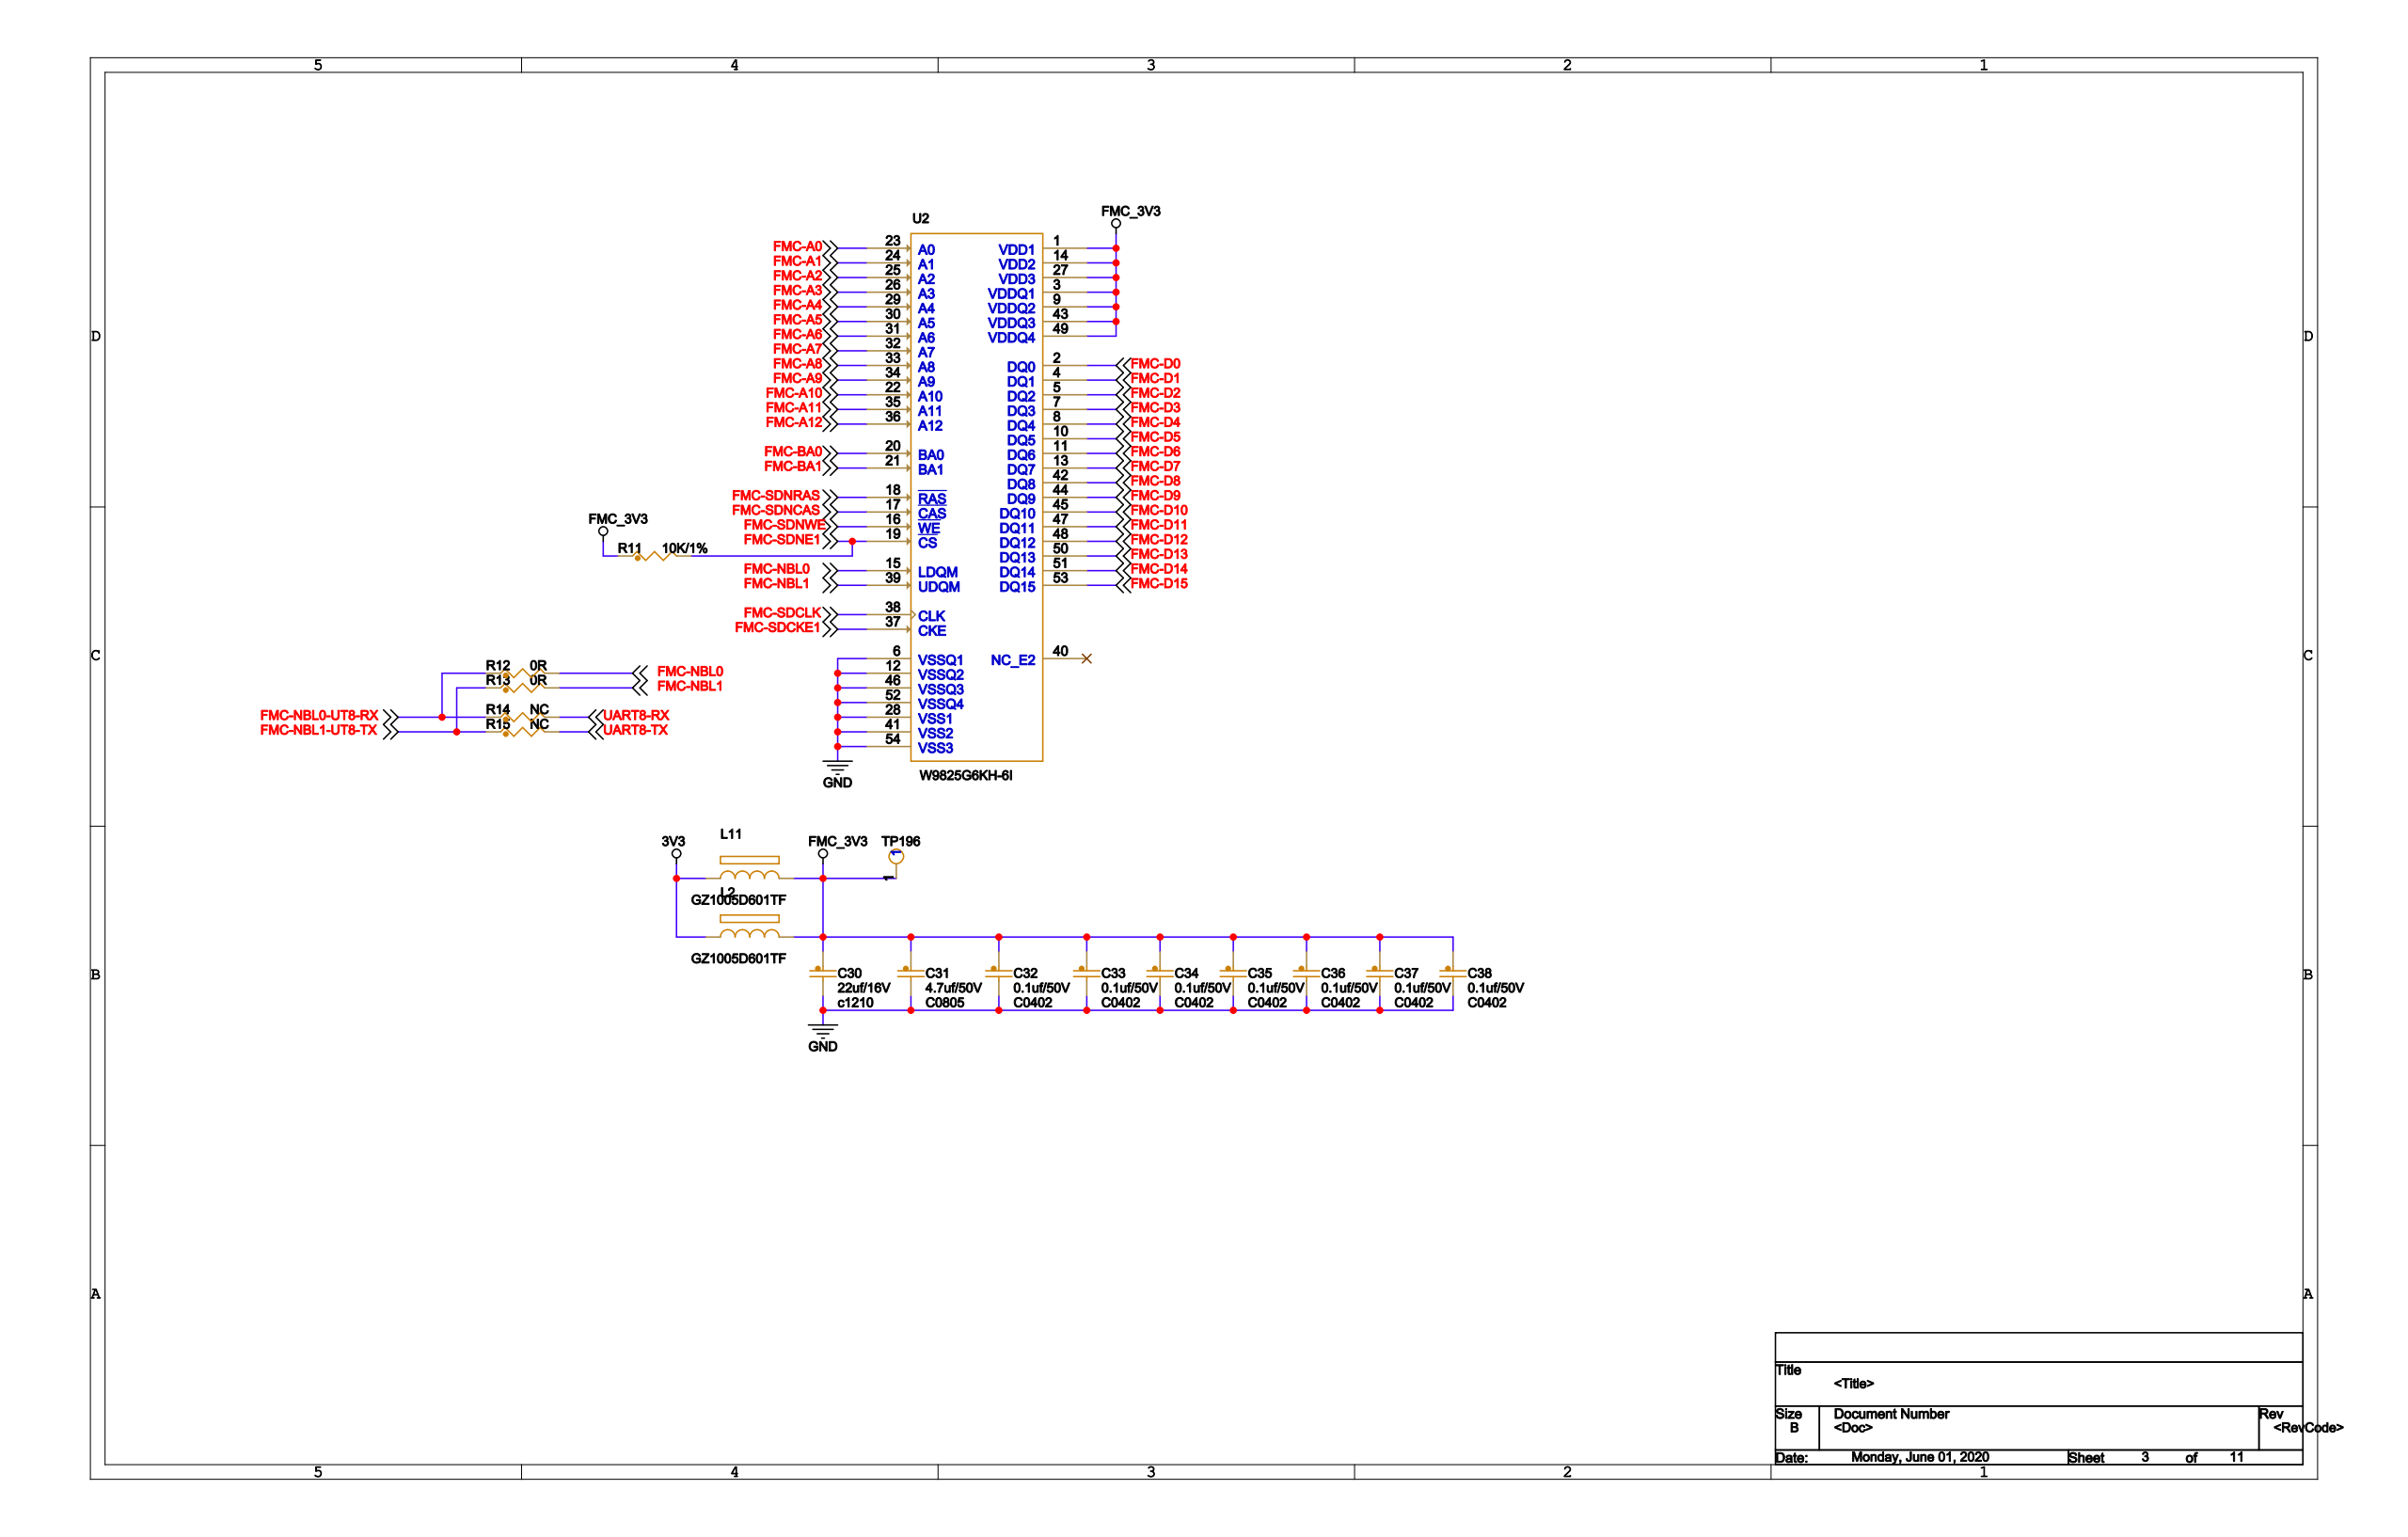Circuit board | Cadence Allegro | 792 parts | 400 nets | one sheet of the schematic
Parts on this sheet (reference | value | footprint):
C30 | 22uf/16V | C1210
C31 | 4.7uf/50V | C0805
C32 | 0.1uf/50V | C0402
C33 | 0.1uf/50V | C0402
C34 | 0.1uf/50V | C0402
C35 | 0.1uf/50V | C0402
C36 | 0.1uf/50V | C0402
C37 | 0.1uf/50V | C0402
C38 | 0.1uf/50V | C0402
L2 | GZ1005D601TF | 0402
L11 | GZ1005D601TF | 0402
R11 | 10K/1% | 0402
R12 | 0R | 0402
R13 | 0R | 0402
R14 | NC | 0402
R15 | NC | 0402
TP196 | TESTPOINT | TESTPOINT-33MIL
U2 | W9825G6KH-6I | TSOP54
Nets of these parts (net: part-pin ...):
FMC-NBL0-UT8-RX: R12-1 R14-1
FMC-NBL0: R12-2 U2-15
FMC-NBL1-UT8-TX: R13-1 R15-1
FMC-NBL1: R13-2 U2-39
3V3: L2-1 L11-1
GND: C30-2 C31-2 C32-2 C33-2 C34-2 C35-2 C36-2 C37-2 C38-2 U2-6 U2-12 U2-28 U2-41 U2-46 U2-52 U2-54
UART8-RX: R14-2
UART8-TX: R15-2
FMC_3V3: C30-1 C31-1 C32-1 C33-1 C34-1 C35-1 C36-1 C37-1 C38-1 L2-2 L11-2 R11-1 TP196-1 U2-1 U2-3 U2-9 U2-14 U2-27 U2-43 U2-49
FMC-SDNE1: R11-2 U2-19
FMC-SDNWE: U2-16
FMC-D2: U2-5
FMC-D3: U2-7
FMC-D15: U2-53
FMC-D0: U2-2
FMC-D1: U2-4
FMC-D13: U2-50
FMC-D14: U2-51
FMC-D7: U2-13
FMC-D8: U2-42
FMC-D9: U2-44
FMC-D10: U2-45
FMC-D11: U2-47
FMC-D12: U2-48
FMC-D4: U2-8
FMC-D5: U2-10
FMC-D6: U2-11
FMC-A0: U2-23
FMC-A1: U2-24
FMC-SDNRAS: U2-18
FMC-A6: U2-31
FMC-A7: U2-32
FMC-A8: U2-33
FMC-A9: U2-34
FMC-A2: U2-25
FMC-A3: U2-26
FMC-A4: U2-29
FMC-A5: U2-30
FMC-A10: U2-22
FMC-A11: U2-35
FMC-SDNCAS: U2-17
FMC-A12: U2-36
FMC-BA0: U2-20
FMC-BA1: U2-21
FMC-SDCLK: U2-38
FMC-SDCKE1: U2-37